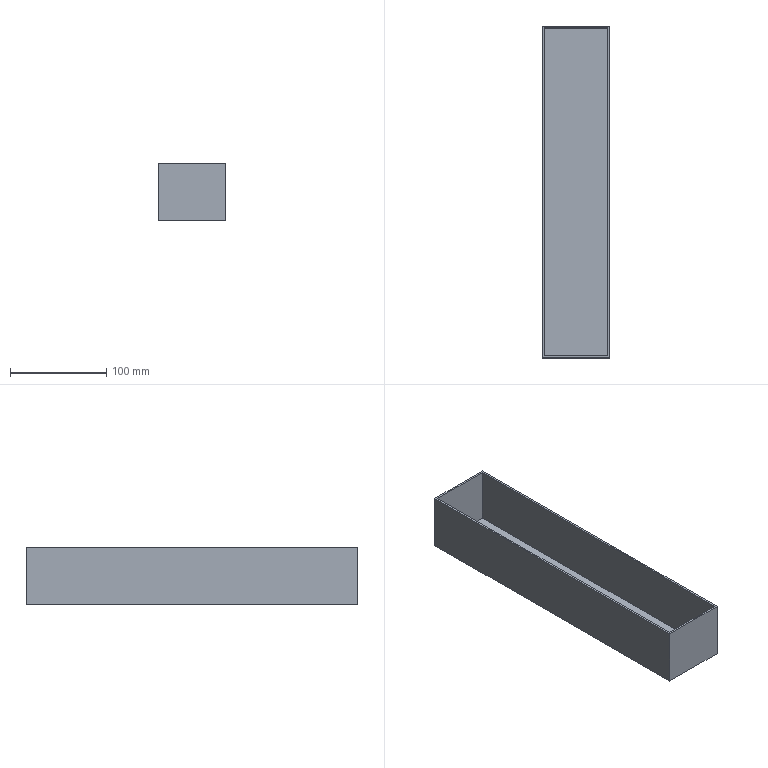Part | NX | features solid 2 | 1 solid | 11 faces | box 70 x 345 x 60 mm | volume 143652 mm3 | plane 11
STEP:
#1=CARTESIAN_POINT('',(-280.,-155.,-255.));
#2=VERTEX_POINT('',#1);
#3=CARTESIAN_POINT('',(-210.,-155.,-255.));
#4=VERTEX_POINT('',#3);
#5=CARTESIAN_POINT('',(-280.,-155.,-255.));
#6=DIRECTION('',(-1.,0.,0.));
#7=VECTOR('',#6,1000.);
#8=LINE('',#5,#7);
#9=EDGE_CURVE('',#2,#4,#8,.F.);
#10=ORIENTED_EDGE('',*,*,#9,.F.);
#11=CARTESIAN_POINT('',(-280.,-500.,-255.));
#12=VERTEX_POINT('',#11);
#13=CARTESIAN_POINT('',(-280.,-155.,-255.));
#14=DIRECTION('',(0.,-1.,0.));
#15=VECTOR('',#14,1000.);
#16=LINE('',#13,#15);
#17=EDGE_CURVE('',#2,#12,#16,.T.);
#18=ORIENTED_EDGE('',*,*,#17,.T.);
#19=CARTESIAN_POINT('',(-210.,-500.,-255.));
#20=VERTEX_POINT('',#19);
#21=CARTESIAN_POINT('',(-280.,-500.,-255.));
#22=DIRECTION('',(-1.,0.,0.));
#23=VECTOR('',#22,1000.);
#24=LINE('',#21,#23);
#25=EDGE_CURVE('',#12,#20,#24,.F.);
#26=ORIENTED_EDGE('',*,*,#25,.T.);
#27=CARTESIAN_POINT('',(-210.,-155.,-255.));
#28=DIRECTION('',(0.,-1.,0.));
#29=VECTOR('',#28,1000.);
#30=LINE('',#27,#29);
#31=EDGE_CURVE('',#4,#20,#30,.T.);
#32=ORIENTED_EDGE('',*,*,#31,.F.);
#33=EDGE_LOOP('',(#10,#18,#26,#32));
#34=FACE_BOUND('',#33,.T.);
#35=CARTESIAN_POINT('',(-278.,-157.,-255.));
#36=VERTEX_POINT('',#35);
#37=CARTESIAN_POINT('',(-278.,-498.,-255.));
#38=VERTEX_POINT('',#37);
#39=CARTESIAN_POINT('',(-278.,-155.,-255.));
#40=DIRECTION('',(0.,-1.,0.));
#41=VECTOR('',#40,1000.);
#42=LINE('',#39,#41);
#43=EDGE_CURVE('',#36,#38,#42,.T.);
#44=ORIENTED_EDGE('',*,*,#43,.F.);
#45=CARTESIAN_POINT('',(-212.,-157.,-255.));
#46=VERTEX_POINT('',#45);
#47=CARTESIAN_POINT('',(-280.,-157.,-255.));
#48=DIRECTION('',(-1.,0.,0.));
#49=VECTOR('',#48,1000.);
#50=LINE('',#47,#49);
#51=EDGE_CURVE('',#36,#46,#50,.F.);
#52=ORIENTED_EDGE('',*,*,#51,.T.);
#53=CARTESIAN_POINT('',(-212.,-498.,-255.));
#54=VERTEX_POINT('',#53);
#55=CARTESIAN_POINT('',(-212.,-155.,-255.));
#56=DIRECTION('',(0.,-1.,0.));
#57=VECTOR('',#56,1000.);
#58=LINE('',#55,#57);
#59=EDGE_CURVE('',#46,#54,#58,.T.);
#60=ORIENTED_EDGE('',*,*,#59,.T.);
#61=CARTESIAN_POINT('',(-280.,-498.,-255.));
#62=DIRECTION('',(-1.,0.,0.));
#63=VECTOR('',#62,1000.);
#64=LINE('',#61,#63);
#65=EDGE_CURVE('',#38,#54,#64,.F.);
#66=ORIENTED_EDGE('',*,*,#65,.F.);
#67=EDGE_LOOP('',(#44,#52,#60,#66));
#68=FACE_BOUND('',#67,.T.);
#69=CARTESIAN_POINT('',(-280.,-155.,-255.));
#70=DIRECTION('',(0.,0.,1.));
#71=DIRECTION('',(0.,-1.,0.));
#72=AXIS2_PLACEMENT_3D('',#69,#70,#71);
#73=PLANE('',#72);
#74=ADVANCED_FACE('',(#34,#68),#73,.T.);
#75=ORIENTED_EDGE('',*,*,#25,.F.);
#76=CARTESIAN_POINT('',(-280.,-500.,-315.));
#77=VERTEX_POINT('',#76);
#78=CARTESIAN_POINT('',(-280.,-500.,-255.));
#79=DIRECTION('',(0.,0.,1.));
#80=VECTOR('',#79,1000.);
#81=LINE('',#78,#80);
#82=EDGE_CURVE('',#12,#77,#81,.F.);
#83=ORIENTED_EDGE('',*,*,#82,.T.);
#84=CARTESIAN_POINT('',(-210.,-500.,-315.));
#85=VERTEX_POINT('',#84);
#86=CARTESIAN_POINT('',(-1080.,-500.,-315.));
#87=DIRECTION('',(1.,0.,0.));
#88=VECTOR('',#87,1000.);
#89=LINE('',#86,#88);
#90=EDGE_CURVE('',#77,#85,#89,.T.);
#91=ORIENTED_EDGE('',*,*,#90,.T.);
#92=CARTESIAN_POINT('',(-210.,-500.,-255.));
#93=DIRECTION('',(0.,0.,1.));
#94=VECTOR('',#93,1000.);
#95=LINE('',#92,#94);
#96=EDGE_CURVE('',#20,#85,#95,.F.);
#97=ORIENTED_EDGE('',*,*,#96,.F.);
#98=EDGE_LOOP('',(#75,#83,#91,#97));
#99=FACE_BOUND('',#98,.T.);
#100=CARTESIAN_POINT('',(-1080.,-500.,-100.));
#101=DIRECTION('',(0.,1.,0.));
#102=DIRECTION('',(0.,0.,1.));
#103=AXIS2_PLACEMENT_3D('',#100,#101,#102);
#104=PLANE('',#103);
#105=ADVANCED_FACE('',(#99),#104,.F.);
#106=ORIENTED_EDGE('',*,*,#90,.F.);
#107=CARTESIAN_POINT('',(-280.,-155.,-315.));
#108=VERTEX_POINT('',#107);
#109=CARTESIAN_POINT('',(-280.,-155.,-315.));
#110=DIRECTION('',(0.,-1.,0.));
#111=VECTOR('',#110,1000.);
#112=LINE('',#109,#111);
#113=EDGE_CURVE('',#108,#77,#112,.T.);
#114=ORIENTED_EDGE('',*,*,#113,.F.);
#115=CARTESIAN_POINT('',(-210.,-155.,-315.));
#116=VERTEX_POINT('',#115);
#117=CARTESIAN_POINT('',(-280.,-155.,-315.));
#118=DIRECTION('',(1.,0.,0.));
#119=VECTOR('',#118,1000.);
#120=LINE('',#117,#119);
#121=EDGE_CURVE('',#108,#116,#120,.T.);
#122=ORIENTED_EDGE('',*,*,#121,.T.);
#123=CARTESIAN_POINT('',(-210.,-155.,-315.));
#124=DIRECTION('',(0.,1.,0.));
#125=VECTOR('',#124,1000.);
#126=LINE('',#123,#125);
#127=EDGE_CURVE('',#116,#85,#126,.F.);
#128=ORIENTED_EDGE('',*,*,#127,.T.);
#129=EDGE_LOOP('',(#106,#114,#122,#128));
#130=FACE_BOUND('',#129,.T.);
#131=CARTESIAN_POINT('',(-280.,-155.,-315.));
#132=DIRECTION('',(0.,0.,1.));
#133=DIRECTION('',(0.,-1.,0.));
#134=AXIS2_PLACEMENT_3D('',#131,#132,#133);
#135=PLANE('',#134);
#136=ADVANCED_FACE('',(#130),#135,.F.);
#137=ORIENTED_EDGE('',*,*,#127,.F.);
#138=CARTESIAN_POINT('',(-210.,-155.,-255.));
#139=DIRECTION('',(0.,0.,1.));
#140=VECTOR('',#139,1000.);
#141=LINE('',#138,#140);
#142=EDGE_CURVE('',#4,#116,#141,.F.);
#143=ORIENTED_EDGE('',*,*,#142,.F.);
#144=ORIENTED_EDGE('',*,*,#31,.T.);
#145=ORIENTED_EDGE('',*,*,#96,.T.);
#146=EDGE_LOOP('',(#137,#143,#144,#145));
#147=FACE_BOUND('',#146,.T.);
#148=CARTESIAN_POINT('',(-210.,-155.,-255.));
#149=DIRECTION('',(1.,0.,0.));
#150=DIRECTION('',(0.,0.,-1.));
#151=AXIS2_PLACEMENT_3D('',#148,#149,#150);
#152=PLANE('',#151);
#153=ADVANCED_FACE('',(#147),#152,.T.);
#154=CARTESIAN_POINT('',(-280.,-155.,-255.));
#155=DIRECTION('',(0.,0.,-1.));
#156=VECTOR('',#155,1000.);
#157=LINE('',#154,#156);
#158=EDGE_CURVE('',#2,#108,#157,.T.);
#159=ORIENTED_EDGE('',*,*,#158,.F.);
#160=ORIENTED_EDGE('',*,*,#9,.T.);
#161=ORIENTED_EDGE('',*,*,#142,.T.);
#162=ORIENTED_EDGE('',*,*,#121,.F.);
#163=EDGE_LOOP('',(#159,#160,#161,#162));
#164=FACE_BOUND('',#163,.T.);
#165=CARTESIAN_POINT('',(-280.,-155.,-255.));
#166=DIRECTION('',(0.,-1.,0.));
#167=DIRECTION('',(0.,0.,-1.));
#168=AXIS2_PLACEMENT_3D('',#165,#166,#167);
#169=PLANE('',#168);
#170=ADVANCED_FACE('',(#164),#169,.F.);
#171=ORIENTED_EDGE('',*,*,#113,.T.);
#172=ORIENTED_EDGE('',*,*,#82,.F.);
#173=ORIENTED_EDGE('',*,*,#17,.F.);
#174=ORIENTED_EDGE('',*,*,#158,.T.);
#175=EDGE_LOOP('',(#171,#172,#173,#174));
#176=FACE_BOUND('',#175,.T.);
#177=CARTESIAN_POINT('',(-280.,-155.,-255.));
#178=DIRECTION('',(1.,0.,0.));
#179=DIRECTION('',(0.,0.,-1.));
#180=AXIS2_PLACEMENT_3D('',#177,#178,#179);
#181=PLANE('',#180);
#182=ADVANCED_FACE('',(#176),#181,.F.);
#183=ORIENTED_EDGE('',*,*,#65,.T.);
#184=CARTESIAN_POINT('',(-212.,-498.,-313.));
#185=VERTEX_POINT('',#184);
#186=CARTESIAN_POINT('',(-212.,-498.,-255.));
#187=DIRECTION('',(0.,0.,1.));
#188=VECTOR('',#187,1000.);
#189=LINE('',#186,#188);
#190=EDGE_CURVE('',#54,#185,#189,.F.);
#191=ORIENTED_EDGE('',*,*,#190,.T.);
#192=CARTESIAN_POINT('',(-278.,-498.,-313.));
#193=VERTEX_POINT('',#192);
#194=CARTESIAN_POINT('',(-1080.,-498.,-313.));
#195=DIRECTION('',(1.,0.,0.));
#196=VECTOR('',#195,1000.);
#197=LINE('',#194,#196);
#198=EDGE_CURVE('',#193,#185,#197,.T.);
#199=ORIENTED_EDGE('',*,*,#198,.F.);
#200=CARTESIAN_POINT('',(-278.,-498.,-255.));
#201=DIRECTION('',(0.,0.,1.));
#202=VECTOR('',#201,1000.);
#203=LINE('',#200,#202);
#204=EDGE_CURVE('',#38,#193,#203,.F.);
#205=ORIENTED_EDGE('',*,*,#204,.F.);
#206=EDGE_LOOP('',(#183,#191,#199,#205));
#207=FACE_BOUND('',#206,.T.);
#208=CARTESIAN_POINT('',(-1080.,-498.,-100.));
#209=DIRECTION('',(0.,1.,0.));
#210=DIRECTION('',(0.,0.,1.));
#211=AXIS2_PLACEMENT_3D('',#208,#209,#210);
#212=PLANE('',#211);
#213=ADVANCED_FACE('',(#207),#212,.T.);
#214=ORIENTED_EDGE('',*,*,#198,.T.);
#215=CARTESIAN_POINT('',(-212.,-157.,-313.));
#216=VERTEX_POINT('',#215);
#217=CARTESIAN_POINT('',(-212.,-155.,-313.));
#218=DIRECTION('',(0.,1.,0.));
#219=VECTOR('',#218,1000.);
#220=LINE('',#217,#219);
#221=EDGE_CURVE('',#216,#185,#220,.F.);
#222=ORIENTED_EDGE('',*,*,#221,.F.);
#223=CARTESIAN_POINT('',(-278.,-157.,-313.));
#224=VERTEX_POINT('',#223);
#225=CARTESIAN_POINT('',(-280.,-157.,-313.));
#226=DIRECTION('',(1.,0.,0.));
#227=VECTOR('',#226,1000.);
#228=LINE('',#225,#227);
#229=EDGE_CURVE('',#224,#216,#228,.T.);
#230=ORIENTED_EDGE('',*,*,#229,.F.);
#231=CARTESIAN_POINT('',(-278.,-155.,-313.));
#232=DIRECTION('',(0.,1.,0.));
#233=VECTOR('',#232,1000.);
#234=LINE('',#231,#233);
#235=EDGE_CURVE('',#224,#193,#234,.F.);
#236=ORIENTED_EDGE('',*,*,#235,.T.);
#237=EDGE_LOOP('',(#214,#222,#230,#236));
#238=FACE_BOUND('',#237,.T.);
#239=CARTESIAN_POINT('',(-280.,-155.,-313.));
#240=DIRECTION('',(0.,0.,1.));
#241=DIRECTION('',(0.,-1.,0.));
#242=AXIS2_PLACEMENT_3D('',#239,#240,#241);
#243=PLANE('',#242);
#244=ADVANCED_FACE('',(#238),#243,.T.);
#245=ORIENTED_EDGE('',*,*,#221,.T.);
#246=ORIENTED_EDGE('',*,*,#190,.F.);
#247=ORIENTED_EDGE('',*,*,#59,.F.);
#248=CARTESIAN_POINT('',(-212.,-157.,-255.));
#249=DIRECTION('',(0.,0.,1.));
#250=VECTOR('',#249,1000.);
#251=LINE('',#248,#250);
#252=EDGE_CURVE('',#46,#216,#251,.F.);
#253=ORIENTED_EDGE('',*,*,#252,.T.);
#254=EDGE_LOOP('',(#245,#246,#247,#253));
#255=FACE_BOUND('',#254,.T.);
#256=CARTESIAN_POINT('',(-212.,-155.,-255.));
#257=DIRECTION('',(1.,0.,0.));
#258=DIRECTION('',(0.,0.,-1.));
#259=AXIS2_PLACEMENT_3D('',#256,#257,#258);
#260=PLANE('',#259);
#261=ADVANCED_FACE('',(#255),#260,.F.);
#262=CARTESIAN_POINT('',(-278.,-157.,-255.));
#263=DIRECTION('',(0.,0.,1.));
#264=VECTOR('',#263,1000.);
#265=LINE('',#262,#264);
#266=EDGE_CURVE('',#36,#224,#265,.F.);
#267=ORIENTED_EDGE('',*,*,#266,.T.);
#268=ORIENTED_EDGE('',*,*,#229,.T.);
#269=ORIENTED_EDGE('',*,*,#252,.F.);
#270=ORIENTED_EDGE('',*,*,#51,.F.);
#271=EDGE_LOOP('',(#267,#268,#269,#270));
#272=FACE_BOUND('',#271,.T.);
#273=CARTESIAN_POINT('',(-280.,-157.,-255.));
#274=DIRECTION('',(0.,-1.,0.));
#275=DIRECTION('',(0.,0.,-1.));
#276=AXIS2_PLACEMENT_3D('',#273,#274,#275);
#277=PLANE('',#276);
#278=ADVANCED_FACE('',(#272),#277,.T.);
#279=ORIENTED_EDGE('',*,*,#235,.F.);
#280=ORIENTED_EDGE('',*,*,#266,.F.);
#281=ORIENTED_EDGE('',*,*,#43,.T.);
#282=ORIENTED_EDGE('',*,*,#204,.T.);
#283=EDGE_LOOP('',(#279,#280,#281,#282));
#284=FACE_BOUND('',#283,.T.);
#285=CARTESIAN_POINT('',(-278.,-155.,-255.));
#286=DIRECTION('',(1.,0.,0.));
#287=DIRECTION('',(0.,0.,-1.));
#288=AXIS2_PLACEMENT_3D('',#285,#286,#287);
#289=PLANE('',#288);
#290=ADVANCED_FACE('',(#284),#289,.T.);
#291=CLOSED_SHELL('',(#74,#105,#136,#153,#170,#182,#213,#244,#261,#278,#290));
#292=MANIFOLD_SOLID_BREP('',#291);
#293=(LENGTH_UNIT()NAMED_UNIT(*)SI_UNIT(.MILLI.,.METRE.));
#294=UNCERTAINTY_MEASURE_WITH_UNIT(LENGTH_MEASURE(0.00001),#293,'','');
#295=(NAMED_UNIT(*)PLANE_ANGLE_UNIT()SI_UNIT($,.RADIAN.));
#296=(NAMED_UNIT(*)SI_UNIT($,.STERADIAN.)SOLID_ANGLE_UNIT());
#297=(GEOMETRIC_REPRESENTATION_CONTEXT(3)GLOBAL_UNCERTAINTY_ASSIGNED_CONTEXT((#294))GLOBAL_UNIT_ASSIGNED_CONTEXT((#293,#295,#296))REPRESENTATION_CONTEXT('',''));
#298=ADVANCED_BREP_SHAPE_REPRESENTATION('',(#292),#297);